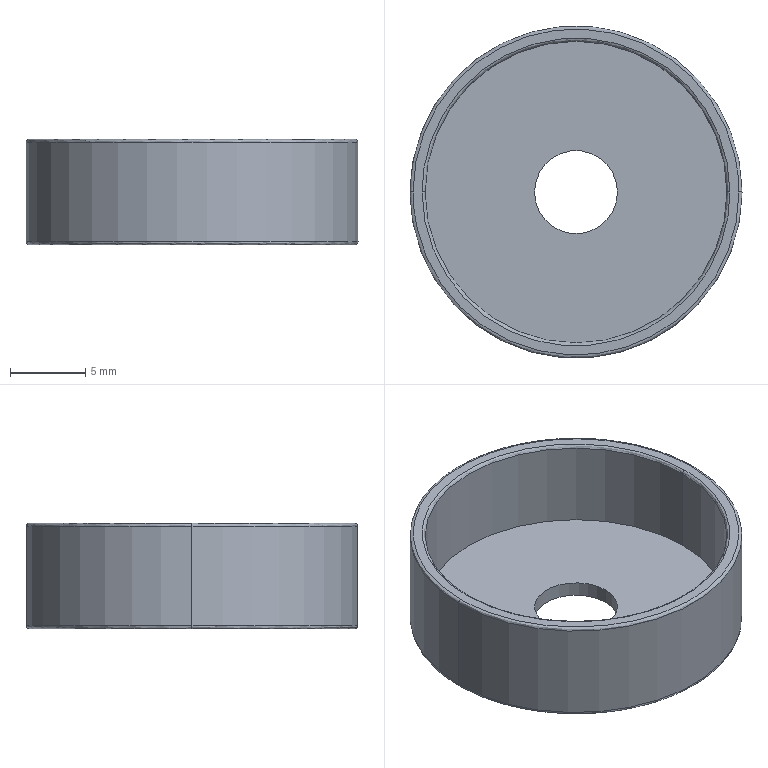Part | STEP file | Rubber buffer pad | 1 solid | 15 faces | box 22 x 22 x 7 mm | volume 750.57 mm3 | spline 6 | cylinder 6 | plane 3 | commonest cylinder face diameters 5.5 x2 20 x2 22 x2